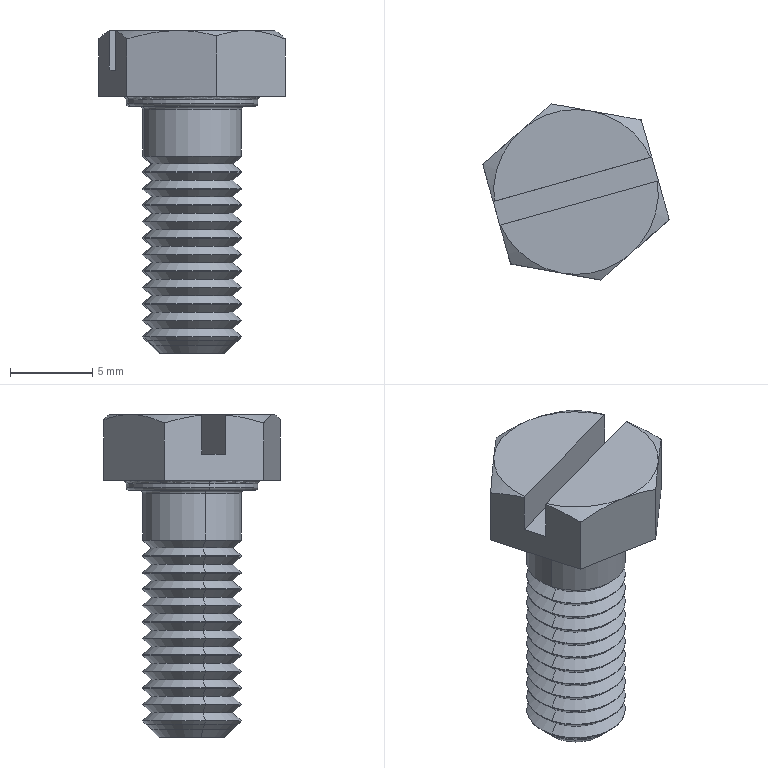Part | SolidWorks | features BaseBody 1 | 1 solid | 108 faces | box 11.322 x 10.694 x 19.6 mm | volume 706.555 mm3 | cone 58 | cylinder 26 | plane 18 | torus 6 | commonest cylinder face diameters 6 x24 8 x2